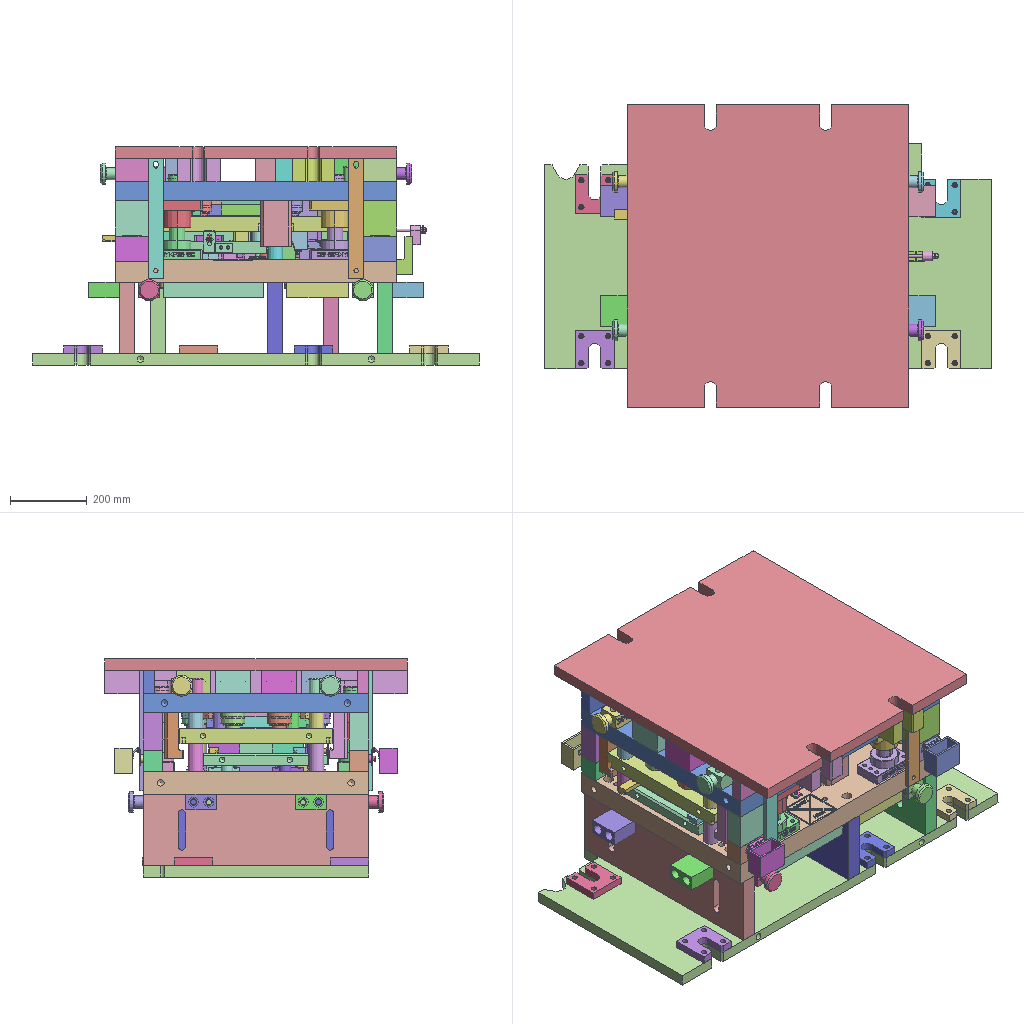Assembly | STEP file | 487 different items | 487 placed | box 1160 x 785 x 567 mm
Parts list (item | name | quantity | size | volume):
1 | 13001_id1154_x_t | x1 | 730 x 585 x 50 mm | 18693036 mm3
2 | 13101_id1802_x_t | x1 | 85 x 30 x 60 mm | 133679 mm3
3 | 13101_id1806_x_t | x1 | 85 x 30 x 60 mm | 133679 mm3
4 | 13101_id1810_x_t | x1 | 85 x 30 x 60 mm | 133679 mm3
5 | 13101_id1814_x_t | x1 | 85 x 30 x 60 mm | 133679 mm3
6 | 13102_id1494_x_t | x1 | 90 x 90 x 60 mm | 430512 mm3
7 | 13102_id1498_x_t | x1 | 90 x 90 x 60 mm | 430512 mm3
8 | 13103_id1506_x_t | x1 | 30 x 90 x 60 mm | 142679 mm3
9 | 13104_id1502_x_t | x1 | 25 x 90 x 60 mm | 115679 mm3
10 | 13105_id1770_x_t | x1 | 112 x 785 x 60 mm | 4657225 mm3
11 | 13106_id1778_x_t | x1 | 90 x 90 x 60 mm | 428886 mm3
12 | 13106_id1782_x_t | x1 | 90 x 90 x 60 mm | 428886 mm3
13 | 13106_id1786_x_t | x1 | 90 x 90 x 60 mm | 428886 mm3
14 | 13106_id1790_x_t | x1 | 90 x 90 x 60 mm | 428886 mm3
15 | 13106_id1794_x_t | x1 | 90 x 90 x 60 mm | 428886 mm3
16 | 13106_id1798_x_t | x1 | 90 x 90 x 60 mm | 428886 mm3
17 | 13107_id1774_x_t | x1 | 110 x 785 x 60 mm | 3912002 mm3
18 | 14001_id1214_x_t | x1 | 40 x 40 x 40 mm | 44485 mm3
19 | 14001_id1218_x_t | x1 | 40 x 40 x 40 mm | 44485 mm3
20 | 14001_id1222_x_t | x1 | 40 x 40 x 40 mm | 44485 mm3
21 | 14001_id1226_x_t | x1 | 40 x 40 x 40 mm | 44485 mm3
22 | 14001_id1230_x_t | x1 | 40 x 40 x 40 mm | 44485 mm3
23 | 14001_id1234_x_t | x1 | 40 x 40 x 40 mm | 44485 mm3
24 | 14001_id1238_x_t | x1 | 40 x 40 x 40 mm | 44485 mm3
25 | 14001_id1242_x_t | x1 | 40 x 40 x 40 mm | 44485 mm3
26 | 14001_id1246_x_t | x1 | 40 x 40 x 40 mm | 44485 mm3
27 | 14001_id1250_x_t | x1 | 40 x 40 x 40 mm | 44485 mm3
28 | 14001_id1254_x_t | x1 | 40 x 40 x 40 mm | 44485 mm3
29 | 14001_id1258_x_t | x1 | 40 x 40 x 40 mm | 44485 mm3
30 | 14001_id1262_x_t | x1 | 40 x 40 x 40 mm | 44485 mm3
31 | 14001_id1266_x_t | x1 | 40 x 40 x 40 mm | 44485 mm3
32 | 14001_id1298_x_t | x1 | 40 x 40 x 40 mm | 44485 mm3
33 | 14001_id1306_x_t | x1 | 40 x 40 x 40 mm | 44485 mm3
34 | 14002_id1738_x_t | x1 | 30.406 x 30.406 x 15 mm | 5664 mm3
35 | 14002_id1742_x_t | x1 | 30.406 x 30.406 x 15 mm | 5664 mm3
36 | 14002_id1746_x_t | x1 | 28.807 x 23.857 x 15 mm | 5664 mm3
37 | 14002_id1750_x_t | x1 | 28.807 x 23.857 x 15 mm | 5664 mm3
38 | 14002_id1754_x_t | x1 | 27.746 x 22.068 x 15 mm | 5664 mm3
39 | 14002_id1758_x_t | x1 | 27.746 x 22.068 x 15 mm | 5664 mm3
40 | 14002_id1762_x_t | x1 | 29.858 x 30.721 x 15 mm | 5664 mm3
41 | 14002_id1766_x_t | x1 | 29.858 x 30.721 x 15 mm | 5664 mm3
42 | 14003_id1942_x_t | x1 | 30 x 16 x 16 mm | 6162 mm3
43 | 14004_id1938_x_t | x1 | 30 x 16 x 16 mm | 6162 mm3
44 | 14101_id882_x_t | x1 | 25 x 40 x 50 mm | 37635 mm3
45 | 14102_id878_x_t | x1 | 25 x 40 x 50 mm | 37635 mm3
46 | 14103_id870_x_t | x1 | 95 x 130 x 28 mm | 241686 mm3
47 | 14104_id886_x_t | x1 | 40 x 25 x 50 mm | 37460 mm3
48 | 14105_id890_x_t | x1 | 90 x 75 x 28 mm | 120807 mm3
49 | 14106_id898_x_t | x1 | 43 x 30 x 50 mm | 41594 mm3
50 | 14107_id966_x_t | x1 | 105 x 120 x 28 mm | 217134 mm3
51 | 14108_id962_x_t | x1 | 105 x 120 x 28 mm | 217134 mm3
52 | 14109_id1038_x_t | x1 | 51 x 55 x 50 mm | 79399 mm3
53 | 14110_id1022_x_t | x1 | 105 x 176 x 28 mm | 281247 mm3
54 | 14111_id1006_x_t | x1 | 51 x 55 x 50 mm | 79567 mm3
55 | 14112_id1034_x_t | x1 | 60 x 85 x 28 mm | 85179 mm3
56 | 14113_id846_x_t | x1 | 727.5 x 395 x 40 mm | 9281090 mm3
57 | 15001_id142_x_t | x1 | 15 x 17 x 108 mm | 21787 mm3
58 | 15002_id766_x_t | x1 | 48.641 x 98 x 108 mm | 278629 mm3
59 | 15003_id762_x_t | x1 | 48.641 x 98 x 108 mm | 278628 mm3
60 | 15004_id854_x_t | x1 | 51.676 x 85.003 x 65 mm | 145640 mm3
61 | 15005_id190_x_t | x1 | 51.676 x 85 x 65 mm | 145641 mm3
62 | 15006_id866_x_t | x1 | 42.5 x 42 x 101 mm | 91343 mm3
63 | 15101_id1058_x_t | x1 | 63.914 x 80 x 35 mm | 137778 mm3
64 | 15102_id758_x_t | x1 | 63.914 x 80 x 35 mm | 137778 mm3
65 | 15103_id754_x_t | x1 | 290 x 208 x 25 mm | 1200558 mm3
66 | 15104_id194_x_t | x1 | 50.466 x 210 x 37 mm | 295873 mm3
67 | 15105_id234_x_t | x1 | 149.23 x 42 x 25 mm | 138214 mm3
68 | 15106_id1078_x_t | x1 | 70 x 85 x 53 mm | 208410 mm3
69 | 15107_id1946_x_t | x1 | 70 x 85 x 53 mm | 208411 mm3
70 | 15108_id850_x_t | x1 | 115 x 175 x 25 mm | 409284 mm3
71 | 16001_id1410_x_t | x1 | 85 x 50 x 97 mm | 372174 mm3
72 | 16001_id1450_x_t | x1 | 85 x 50 x 97 mm | 372174 mm3
73 | 16001_id1466_x_t | x1 | 85 x 50 x 97 mm | 372174 mm3
74 | 16001_id1482_x_t | x1 | 85 x 50 x 97 mm | 372174 mm3
75 | 16002_id1274_x_t | x1 | 80 x 50 x 118 mm | 264145 mm3
76 | 16002_id1278_x_t | x1 | 80 x 50 x 118 mm | 264145 mm3
77 | 16002_id1282_x_t | x1 | 80 x 50 x 118 mm | 264145 mm3
78 | 16002_id1286_x_t | x1 | 80 x 50 x 118 mm | 264145 mm3
79 | 16002_id1290_x_t | x1 | 80 x 50 x 118 mm | 264145 mm3
80 | 16002_id1294_x_t | x1 | 80 x 50 x 118 mm | 264145 mm3
81 | 16003_id874_x_t | x1 | 95 x 130 x 10 mm | 115889 mm3
82 | 16004_id894_x_t | x1 | 90 x 75 x 10 mm | 57234 mm3
83 | 16005_id970_x_t | x1 | 105 x 120 x 10 mm | 118397 mm3
84 | 16005_id974_x_t | x1 | 105 x 120 x 10 mm | 118397 mm3
85 | 16006_id862_x_t | x1 | 74.676 x 85 x 110 mm | 490058 mm3
86 | 16007_id858_x_t | x1 | 74.676 x 85 x 110 mm | 490062 mm3
87 | 16008_id1026_x_t | x1 | 105 x 176 x 10 mm | 142706 mm3
88 | 16009_id1030_x_t | x1 | 60 x 85 x 10 mm | 42512 mm3
89 | 6-35_id1850_x_t | x1 | 8 x 8 x 38 mm | 1137 mm3
90 | 6-35_id1870_x_t | x1 | 8 x 8 x 38 mm | 1137 mm3
91 | - | x1 | 94 x 140 x 15 mm | 130830 mm3
92 | - | x1 | 58 x 85.001 x 56.5 mm | 200915 mm3
93 | - | x1 | 30 x 30 x 27 mm | 14276 mm3
94 | - | x1 | 30 x 30 x 27 mm | 14276 mm3
95 | - | x1 | 30 x 30 x 27 mm | 14276 mm3
96 | - | x1 | 26.045 x 93.231 x 17.45 mm | 4101 mm3
97 | - | x1 | 30 x 30 x 27 mm | 14276 mm3
98 | - | x1 | 40 x 40 x 72 mm | 79413 mm3
99 | - | x1 | 40 x 40 x 72 mm | 79413 mm3
100 | - | x1 | 40 x 40 x 72 mm | 79413 mm3
101 | - | x1 | 40 x 40 x 72 mm | 79413 mm3
102 | - | x1 | 99 x 140 x 30 mm | 280871 mm3
103 | - | x1 | 40 x 40 x 72 mm | 79413 mm3
104 | - | x1 | 99 x 140 x 15 mm | 135777 mm3
105 | - | x1 | 40 x 40 x 72 mm | 79413 mm3
106 | - | x1 | 42 x 25 x 98 mm | 60681 mm3
107 | - | x1 | 40 x 585 x 185 mm | 4078797 mm3
108 | - | x1 | 40 x 585 x 185 mm | 4012325 mm3
109 | - | x1 | 100 x 100 x 20 mm | 150755 mm3
110 | - | x1 | 100 x 100 x 20 mm | 150755 mm3
111 | - | x1 | 100 x 100 x 20 mm | 150755 mm3
112 | - | x1 | 40 x 255 x 185 mm | 1855337 mm3
113 | - | x1 | 40 x 255 x 185 mm | 1874377 mm3
114 | - | x1 | 40 x 585 x 185 mm | 4281820 mm3
115 | - | x1 | 85 x 50 x 55 mm | 210302 mm3
116 | - | x1 | 85 x 74 x 66.5 mm | 93814 mm3
117 | - | x1 | 85 x 50 x 55 mm | 210302 mm3
118 | - | x1 | 85 x 74 x 66.5 mm | 93814 mm3
119 | - | x1 | 85 x 50 x 55 mm | 210302 mm3
120 | - | x1 | 63 x 73 x 30 mm | 93374 mm3
121 | - | x1 | 85 x 74 x 66.5 mm | 93814 mm3
122 | - | x1 | 85 x 50 x 55 mm | 210302 mm3
123 | - | x1 | 85 x 74 x 66.5 mm | 93814 mm3
124 | - | x1 | 60 x 80 x 56.5 mm | 99207 mm3
125 | - | x1 | 28 x 43 x 30 mm | 25680 mm3
126 | - | x1 | 63 x 73 x 15 mm | 59595 mm3
127 | - | x1 | 30 x 30 x 15 mm | 8745 mm3
128 | - | x1 | 30 x 30 x 15 mm | 8745 mm3
129 | - | x1 | 30 x 30 x 15 mm | 8745 mm3
130 | - | x1 | 30 x 30 x 15 mm | 8745 mm3
131 | - | x1 | 30 x 30 x 15 mm | 8745 mm3
132 | - | x1 | 105 x 25 x 16 mm | 33608 mm3
133 | - | x1 | 45 x 25 x 16 mm | 13030 mm3
134 | - | x1 | 90 x 25 x 80 mm | 146448 mm3
135 | - | x1 | 90 x 25 x 80 mm | 146448 mm3
136 | - | x1 | 80 x 80 x 40 mm | 195367 mm3
137 | - | x1 | 80 x 80 x 40 mm | 195367 mm3
138 | - | x1 | 80 x 80 x 40 mm | 195367 mm3
139 | - | x1 | 80 x 80 x 40 mm | 195367 mm3
140 | - | x1 | 19.63 x 48.1 x 17 mm | 5552 mm3
141 | - | x1 | 75 x 27 x 53.7 mm | 8311 mm3
142 | - | x1 | 65 x 48 x 16 mm | 32002 mm3
143 | - | x1 | 15 x 70.5 x 16 mm | 11235 mm3
144 | - | x1 | 1160 x 585 x 30 mm | 18789042 mm3
145 | - | x1 | 100 x 100 x 20 mm | 150755 mm3
146 | - | x1 | 100 x 100 x 20 mm | 150755 mm3
147 | - | x1 | 19.1 x 19.1 x 30 mm | 8502 mm3
148 | - | x1 | 260 x 40 x 40 mm | 385684 mm3
149 | - | x1 | 260 x 40 x 40 mm | 385684 mm3
150 | - | x1 | 160 x 40 x 40 mm | 225684 mm3
151 | - | x1 | 160 x 40 x 40 mm | 225684 mm3
152 | - | x1 | 100 x 100 x 20 mm | 150755 mm3
153 | - | x1 | 40 x 10 x 317 mm | 124006 mm3
154 | - | x1 | 40 x 10 x 317 mm | 124006 mm3
155 | - | x1 | 40 x 10 x 317 mm | 124006 mm3
156 | - | x1 | 40 x 10 x 317 mm | 124006 mm3
157 | - | x1 | 58.148 x 85 x 56.5 mm | 200916 mm3
158 | - | x1 | 58 x 85 x 56.501 mm | 217515 mm3
159 | - | x1 | 40 x 55 x 53 mm | 73845 mm3
160 | - | x1 | - | 214872 mm3
161 | - | x1 | 65 x 75 x 45.001 mm | 106035 mm3
162 | - | x1 | 19 x 17 x 20 mm | 5075 mm3
163 | - | x1 | 15 x 13 x 20 mm | 2634 mm3
164 | - | x1 | 13.98 x 12 x 20 mm | 2357 mm3
165 | - | x1 | 23.1 x 23.1 x 30 mm | 13334 mm3
166 | - | x1 | 80 x 90 x 30 mm | 141495 mm3
167 | - | x1 | 80 x 90 x 15 mm | 69642 mm3
168 | - | x1 | 70 x 120 x 30 mm | 188611 mm3
169 | - | x1 | 40 x 55 x 53 mm | 73845 mm3
170 | - | x1 | 58 x 85 x 56.501 mm | 217785 mm3
171 | - | x1 | 70 x 120 x 15 mm | 114867 mm3
172 | - | x1 | 58.914 x 80 x 15 mm | 42146 mm3
173 | - | x1 | 19.1 x 19.1 x 30 mm | 8502 mm3
174 | - | x1 | 60 x 80 x 56.5 mm | 99206 mm3
175 | - | x1 | 58.914 x 80 x 15 mm | 42146 mm3
176 | - | x1 | 105 x 25 x 16 mm | 33608 mm3
177 | - | x1 | 70 x 33 x 16 mm | 29565 mm3
178 | - | x1 | 20 x 25 x 7 mm | 3055 mm3
179 | - | x1 | 20 x 25 x 7 mm | 3055 mm3
180 | - | x1 | 20 x 25 x 7 mm | 3055 mm3
181 | - | x1 | 25 x 20 x 7 mm | 3055 mm3
182 | - | x1 | 730 x 585 x 60 mm | 23773121 mm3
183 | - | x1 | 240 x 52 x 30 mm | 250447 mm3
184 | - | x1 | 65 x 75 x 45.001 mm | 106042 mm3
185 | - | x1 | 19 x 17 x 20 mm | 5075 mm3
186 | - | x1 | 15 x 13 x 20 mm | 2634 mm3
187 | - | x1 | 13.98 x 12 x 20 mm | 2357 mm3
188 | - | x1 | 730 x 785 x 30 mm | 16951245 mm3
189 | - | x1 | 20 x 25 x 7 mm | 3055 mm3
190 | - | x1 | 25 x 20 x 7 mm | 3055 mm3
191 | - | x1 | 94 x 140 x 30 mm | 271163 mm3
192 | - | x1 | 400 x 325 x 30 mm | 2323925 mm3
193 | CB-_id1538_x_t | x1 | 16 x 16 x 50 mm | 4584 mm3
194 | CB-_id1542_x_t | x1 | 16 x 16 x 50 mm | 4584 mm3
195 | CB-_id1558_x_t | x1 | 16 x 16 x 50 mm | 4584 mm3
196 | CB-_id1562_x_t | x1 | 16 x 16 x 50 mm | 4584 mm3
197 | CHP10_id1818_x_t | x1 | 118 x 55 x 55 mm | 202286 mm3
198 | CHP10_id1822_x_t | x1 | 118 x 55 x 55 mm | 202286 mm3
199 | CHP10_id1826_x_t | x1 | 118 x 55 x 55 mm | 202286 mm3
200 | CHP10_id1830_x_t | x1 | 118 x 55 x 55 mm | 202286 mm3
201 | CHP10_id1834_x_t | x1 | 55 x 118 x 55 mm | 202286 mm3
202 | CHP10_id1838_x_t | x1 | 55 x 118 x 55 mm | 202286 mm3
203 | CHP10_id1842_x_t | x1 | 55 x 118 x 55 mm | 202286 mm3
204 | CHP10_id1846_x_t | x1 | 55 x 118 x 55 mm | 202286 mm3
205 | D10-50_id1526_x_t | x1 | 10 x 10 x 50 mm | 3878 mm3
206 | D10-50_id1546_x_t | x1 | 10 x 10 x 50 mm | 3878 mm3
207 | D10-50_id1566_x_t | x1 | 10 x 10 x 50 mm | 3878 mm3
208 | D8-50_id110_x_t | x1 | 10 x 10 x 50 mm | 3919 mm3
209 | D8-50_id114_x_t | x1 | 10 x 10 x 50 mm | 3919 mm3
210 | D8-50_id118_x_t | x1 | 10 x 10 x 50 mm | 3919 mm3
211 | D8-50_id122_x_t | x1 | 10 x 10 x 50 mm | 3919 mm3
212 | D8-50_id1614_x_t | x1 | 8 x 8 x 30 mm | 1502 mm3
213 | D8-50_id1622_x_t | x1 | 8 x 8 x 30 mm | 1502 mm3
214 | D8-50_id1634_x_t | x1 | 8 x 8 x 30 mm | 1502 mm3
215 | D8-50_id1642_x_t | x1 | 8 x 8 x 30 mm | 1502 mm3
216 | D8-50_id1654_x_t | x1 | 8 x 8 x 30 mm | 1502 mm3
217 | D8-50_id1658_x_t | x1 | 8 x 8 x 30 mm | 1502 mm3
218 | D8-50_id1662_x_t | x1 | 8 x 8 x 30 mm | 1502 mm3
219 | D8-50_id166_x_t | x1 | 8 x 8 x 45 mm | 2256 mm3
220 | D8-50_id1674_x_t | x1 | 8 x 8 x 30 mm | 1502 mm3
221 | D8-50_id1686_x_t | x1 | 8 x 8 x 30 mm | 1502 mm3
222 | D8-50_id1690_x_t | x1 | 8 x 8 x 30 mm | 1502 mm3
223 | D8-50_id170_x_t | x1 | 8 x 8 x 45 mm | 2256 mm3
224 | D8-50_id294_x_t | x1 | 8 x 8 x 30 mm | 1502 mm3
225 | D8-50_id298_x_t | x1 | 8 x 8 x 30 mm | 1502 mm3
226 | D8-50_id354_x_t | x1 | 8 x 8 x 45 mm | 2256 mm3
227 | D8-50_id362_x_t | x1 | 8 x 8 x 45 mm | 2256 mm3
228 | D8-50_id394_x_t | x1 | 8 x 8 x 30 mm | 1502 mm3
229 | D8-50_id398_x_t | x1 | 8 x 8 x 30 mm | 1502 mm3
230 | D8-50_id406_x_t | x1 | 10 x 10 x 40 mm | 3134 mm3
231 | D8-50_id410_x_t | x1 | 8 x 8 x 30 mm | 1502 mm3
232 | D8-50_id426_x_t | x1 | 8 x 8 x 30 mm | 1502 mm3
233 | D8-50_id446_x_t | x1 | 10 x 10 x 40 mm | 3134 mm3
234 | D8-50_id474_x_t | x1 | 8 x 8 x 30 mm | 1502 mm3
235 | D8-50_id478_x_t | x1 | 8 x 8 x 30 mm | 1502 mm3
236 | D8-50_id486_x_t | x1 | 8 x 8 x 30 mm | 1502 mm3
237 | D8-50_id490_x_t | x1 | 8 x 8 x 30 mm | 1502 mm3
238 | D8-50_id54_x_t | x1 | 10 x 10 x 50 mm | 3919 mm3
239 | D8-50_id622_x_t | x1 | 8 x 8 x 30 mm | 1502 mm3
240 | D8-50_id626_x_t | x1 | 8 x 8 x 30 mm | 1502 mm3
241 | D8-50_id62_x_t | x1 | 10 x 10 x 50 mm | 3919 mm3
242 | D8-50_id82_x_t | x1 | 10 x 10 x 40 mm | 3134 mm3
243 | D8-50_id86_x_t | x1 | 10 x 10 x 40 mm | 3134 mm3
244 | GSV170-7_id1158_x_t | x1 | 50 x 50 x 114 mm | 158224 mm3
245 | GSV170-7_id1162_x_t | x1 | 50 x 50 x 114 mm | 158224 mm3
246 | GSV170-7_id1166_x_t | x1 | 50 x 50 x 114 mm | 158224 mm3
247 | GSV170-7_id1170_x_t | x1 | 50 x 50 x 114 mm | 158224 mm3
248 | GSV170-7_id1174_x_t | x1 | 50 x 50 x 114 mm | 158224 mm3
249 | GSV170-7_id1178_x_t | x1 | 50 x 50 x 114 mm | 158224 mm3
250 | GSV170-7_id1182_x_t | x1 | 63 x 63 x 120 mm | 273871 mm3
251 | GSV170-7_id1186_x_t | x1 | 63 x 63 x 120 mm | 273871 mm3
252 | GSV170-7_id1190_x_t | x1 | 63 x 63 x 120 mm | 273871 mm3
253 | GSV170-7_id1194_x_t | x1 | 63 x 63 x 120 mm | 273871 mm3
254 | GSV170-7_id1270_x_t | x1 | 50 x 50 x 114 mm | 158224 mm3
255 | GSV170-7_id506_x_t | x1 | 19 x 19 x 106 mm | 21365 mm3
256 | GSV170-7_id514_x_t | x1 | 19 x 19 x 106 mm | 21365 mm3
257 | GSV170-7_id530_x_t | x1 | 19 x 19 x 106 mm | 21365 mm3
258 | GSV170-7_id550_x_t | x1 | 19 x 19 x 106 mm | 21365 mm3
259 | GSV170-7_id670_x_t | x1 | 19 x 19 x 106 mm | 21365 mm3
260 | GSV170-7_id734_x_t | x1 | 19 x 19 x 106 mm | 21365 mm3
261 | LPS 2-10_id1002_x_t | x1 | 8 x 8 x 60 mm | 2567 mm3
262 | LPS 2-10_id1010_x_t | x1 | 8 x 8 x 60 mm | 2567 mm3
263 | LPS 2-10_id1014_x_t | x1 | 8 x 8 x 60 mm | 2567 mm3
264 | LPS 2-10_id1018_x_t | x1 | 8 x 8 x 60 mm | 2567 mm3
265 | LPS 2-10_id1042_x_t | x1 | 8 x 8 x 60 mm | 2567 mm3
266 | LPS 2-10_id1046_x_t | x1 | 8 x 8 x 60 mm | 2567 mm3
267 | LPS 2-10_id1050_x_t | x1 | 8 x 8 x 60 mm | 2567 mm3
268 | LPS 2-10_id1054_x_t | x1 | 8 x 8 x 60 mm | 2567 mm3
269 | LPS 2-10_id902_x_t | x1 | 8 x 8 x 60 mm | 2567 mm3
270 | LPS 2-10_id906_x_t | x1 | 8 x 8 x 60 mm | 2567 mm3
271 | LPS 2-10_id910_x_t | x1 | 8 x 8 x 60 mm | 2567 mm3
272 | LPS 2-10_id914_x_t | x1 | 8 x 8 x 60 mm | 2567 mm3
273 | LPS 2-10_id918_x_t | x1 | 8 x 8 x 60 mm | 2567 mm3
274 | LPS 2-10_id922_x_t | x1 | 8 x 8 x 60 mm | 2567 mm3
275 | LPS 2-10_id926_x_t | x1 | 8 x 8 x 60 mm | 2567 mm3
276 | LPS 2-10_id930_x_t | x1 | 8 x 8 x 60 mm | 2567 mm3
277 | LPS 2-10_id934_x_t | x1 | 8 x 8 x 60 mm | 2567 mm3
278 | LPS 2-10_id938_x_t | x1 | 8 x 8 x 60 mm | 2567 mm3
279 | LPS 2-10_id942_x_t | x1 | 8 x 8 x 60 mm | 2567 mm3
280 | LPS 2-10_id946_x_t | x1 | 8 x 8 x 60 mm | 2567 mm3
281 | LPS 2-10_id950_x_t | x1 | 8 x 8 x 60 mm | 2567 mm3
282 | LPS 2-10_id954_x_t | x1 | 8 x 8 x 60 mm | 2567 mm3
283 | LPS 2-10_id958_x_t | x1 | 8 x 8 x 60 mm | 2567 mm3
284 | LPS 2-10_id978_x_t | x1 | 8 x 8 x 60 mm | 2567 mm3
285 | LPS 2-10_id982_x_t | x1 | 8 x 8 x 60 mm | 2567 mm3
286 | LPS 2-10_id986_x_t | x1 | 8 x 8 x 60 mm | 2567 mm3
287 | LPS 2-10_id990_x_t | x1 | 8 x 8 x 60 mm | 2567 mm3
288 | LPS 2-10_id994_x_t | x1 | 8 x 8 x 60 mm | 2567 mm3
289 | LPS 2-10_id998_x_t | x1 | 8 x 8 x 60 mm | 2567 mm3
290 | M3-10_id102_x_t | x1 | 16 x 16 x 55 mm | 4808 mm3
291 | M3-10_id134_x_t | x1 | 16 x 16 x 55 mm | 4808 mm3
292 | M3-10_id1370_x_t | x1 | 43 x 13 x 13 mm | 2482 mm3
293 | M3-10_id138_x_t | x1 | 16 x 16 x 55 mm | 4808 mm3
294 | M3-10_id1418_x_t | x1 | 16 x 16 x 45 mm | 4022 mm3
295 | M3-10_id1422_x_t | x1 | 16 x 16 x 45 mm | 4022 mm3
296 | M3-10_id1426_x_t | x1 | 13 x 33 x 13 mm | 1987 mm3
297 | M3-10_id1430_x_t | x1 | 13 x 33 x 13 mm | 1987 mm3
298 | M3-10_id1438_x_t | x1 | 16 x 16 x 45 mm | 4022 mm3
299 | M3-10_id1442_x_t | x1 | 13 x 33 x 13 mm | 1987 mm3
300 | M3-10_id1446_x_t | x1 | 13 x 33 x 13 mm | 1987 mm3
301 | M3-10_id1458_x_t | x1 | 16 x 16 x 45 mm | 4022 mm3
302 | M3-10_id1478_x_t | x1 | 16 x 16 x 45 mm | 4022 mm3
303 | M3-10_id1490_x_t | x1 | 16 x 16 x 45 mm | 4022 mm3
304 | M3-10_id1574_x_t | x1 | 13 x 13 x 28 mm | 1728 mm3
305 | M3-10_id1582_x_t | x1 | 13 x 13 x 28 mm | 1728 mm3
306 | M3-10_id1586_x_t | x1 | 13 x 13 x 28 mm | 1728 mm3
307 | M3-10_id158_x_t | x1 | 13 x 13 x 48 mm | 2734 mm3
308 | M3-10_id1598_x_t | x1 | 13 x 13 x 28 mm | 1728 mm3
309 | M3-10_id1606_x_t | x1 | 13 x 13 x 28 mm | 1728 mm3
310 | M3-10_id1618_x_t | x1 | 13 x 13 x 28 mm | 1742 mm3
311 | M3-10_id1626_x_t | x1 | 13 x 13 x 28 mm | 1742 mm3
312 | M3-10_id162_x_t | x1 | 13 x 13 x 48 mm | 2734 mm3
313 | M3-10_id1638_x_t | x1 | 13 x 13 x 28 mm | 1742 mm3
314 | M3-10_id1650_x_t | x1 | 13 x 13 x 48 mm | 2734 mm3
315 | M3-10_id1666_x_t | x1 | 13 x 13 x 48 mm | 2734 mm3
316 | M3-10_id1678_x_t | x1 | 13 x 13 x 28 mm | 1742 mm3
317 | M3-10_id1682_x_t | x1 | 13 x 13 x 28 mm | 1742 mm3
318 | M3-10_id210_x_t | x1 | 20 x 8.5 x 8.5 mm | 482.387 mm3
319 | M3-10_id214_x_t | x1 | 20 x 8.5 x 8.5 mm | 482.387 mm3
320 | M3-10_id218_x_t | x1 | 16 x 16 x 40 mm | 3630 mm3
321 | M3-10_id222_x_t | x1 | 16 x 16 x 40 mm | 3630 mm3
322 | M3-10_id226_x_t | x1 | 16 x 16 x 40 mm | 3630 mm3
323 | M3-10_id230_x_t | x1 | 16 x 16 x 40 mm | 3630 mm3
324 | M3-10_id238_x_t | x1 | 16 x 16 x 40 mm | 3630 mm3
325 | M3-10_id242_x_t | x1 | 16 x 16 x 40 mm | 3630 mm3
326 | M3-10_id262_x_t | x1 | 8.5 x 8.5 x 20 mm | 456.375 mm3
327 | M3-10_id266_x_t | x1 | 8.5 x 8.5 x 20 mm | 456.375 mm3
328 | M3-10_id270_x_t | x1 | 8.5 x 8.5 x 20 mm | 456.375 mm3
329 | M3-10_id278_x_t | x1 | 10 x 10 x 46 mm | 1459 mm3
330 | M3-10_id282_x_t | x1 | 13 x 13 x 33 mm | 1980 mm3
331 | M3-10_id286_x_t | x1 | 13 x 13 x 33 mm | 1980 mm3
332 | M3-10_id290_x_t | x1 | 13 x 13 x 33 mm | 1980 mm3
333 | M3-10_id306_x_t | x1 | 20 x 8.5 x 8.5 mm | 482.387 mm3
334 | M3-10_id310_x_t | x1 | 16 x 16 x 40 mm | 3630 mm3
335 | M3-10_id314_x_t | x1 | 16 x 16 x 40 mm | 3630 mm3
336 | M3-10_id318_x_t | x1 | 20 x 8.5 x 8.5 mm | 482.387 mm3
337 | M3-10_id322_x_t | x1 | 16 x 16 x 40 mm | 3630 mm3
338 | M3-10_id326_x_t | x1 | 16 x 16 x 40 mm | 3630 mm3
339 | M3-10_id338_x_t | x1 | 16 x 16 x 40 mm | 3630 mm3
340 | M3-10_id346_x_t | x1 | 16 x 16 x 40 mm | 3630 mm3
341 | M3-10_id350_x_t | x1 | 13 x 13 x 48 mm | 2734 mm3
342 | M3-10_id358_x_t | x1 | 13 x 13 x 48 mm | 2734 mm3
343 | M3-10_id374_x_t | x1 | 8.5 x 8.5 x 20 mm | 456.375 mm3
344 | M3-10_id378_x_t | x1 | 13 x 13 x 28 mm | 1728 mm3
345 | M3-10_id382_x_t | x1 | 13 x 13 x 28 mm | 1728 mm3
346 | M3-10_id386_x_t | x1 | 13 x 13 x 28 mm | 1728 mm3
347 | M3-10_id38_x_t | x1 | 8.5 x 8.5 x 20 mm | 456.375 mm3
348 | M3-10_id390_x_t | x1 | 13 x 13 x 28 mm | 1728 mm3
349 | M3-10_id402_x_t | x1 | 13 x 13 x 28 mm | 1728 mm3
350 | M3-10_id414_x_t | x1 | 13 x 13 x 33 mm | 1980 mm3
351 | M3-10_id418_x_t | x1 | 13 x 13 x 33 mm | 1980 mm3
352 | M3-10_id422_x_t | x1 | 13 x 13 x 28 mm | 1728 mm3
353 | M3-10_id42_x_t | x1 | 8.5 x 8.5 x 20 mm | 456.375 mm3
354 | M3-10_id434_x_t | x1 | 13 x 13 x 33 mm | 1980 mm3
355 | M3-10_id442_x_t | x1 | 13 x 13 x 28 mm | 1728 mm3
356 | M3-10_id450_x_t | x1 | 13 x 13 x 28 mm | 1728 mm3
357 | M3-10_id454_x_t | x1 | 13 x 13 x 33 mm | 1980 mm3
358 | M3-10_id466_x_t | x1 | 13 x 13 x 28 mm | 1742 mm3
359 | M3-10_id46_x_t | x1 | 16 x 16 x 55 mm | 4808 mm3
360 | M3-10_id470_x_t | x1 | 13 x 13 x 28 mm | 1742 mm3
361 | M3-10_id482_x_t | x1 | 13 x 13 x 28 mm | 1742 mm3
362 | M3-10_id50_x_t | x1 | 16 x 16 x 55 mm | 4808 mm3
363 | M3-10_id566_x_t | x1 | 10 x 10 x 26 mm | 877.848 mm3
364 | M3-10_id570_x_t | x1 | 10 x 10 x 26 mm | 877.848 mm3
365 | M3-10_id574_x_t | x1 | 10 x 10 x 26 mm | 877.848 mm3
366 | M3-10_id578_x_t | x1 | 10 x 10 x 26 mm | 877.848 mm3
367 | M3-10_id582_x_t | x1 | 10 x 10 x 26 mm | 877.848 mm3
368 | M3-10_id586_x_t | x1 | 10 x 10 x 26 mm | 877.848 mm3
369 | M3-10_id58_x_t | x1 | 16 x 16 x 55 mm | 4808 mm3
370 | M3-10_id590_x_t | x1 | 10 x 10 x 26 mm | 877.848 mm3
371 | M3-10_id594_x_t | x1 | 10 x 10 x 26 mm | 877.848 mm3
372 | M3-10_id598_x_t | x1 | 13 x 13 x 28 mm | 1756 mm3
373 | M3-10_id602_x_t | x1 | 13 x 13 x 28 mm | 1756 mm3
374 | M3-10_id606_x_t | x1 | 13 x 13 x 28 mm | 1756 mm3
375 | M3-10_id614_x_t | x1 | 8.5 x 8.5 x 20 mm | 456.375 mm3
376 | M3-10_id630_x_t | x1 | 13 x 13 x 33 mm | 1980 mm3
377 | M3-10_id634_x_t | x1 | 8.5 x 8.5 x 20 mm | 456.375 mm3
378 | M3-10_id638_x_t | x1 | 8.5 x 8.5 x 20 mm | 456.375 mm3
379 | M3-10_id646_x_t | x1 | 13 x 13 x 33 mm | 1980 mm3
380 | M3-10_id658_x_t | x1 | 13 x 13 x 33 mm | 1980 mm3
381 | M3-10_id662_x_t | x1 | 10 x 10 x 26 mm | 877.848 mm3
382 | M3-10_id666_x_t | x1 | 10 x 10 x 26 mm | 877.848 mm3
383 | M3-10_id66_x_t | x1 | 13 x 13 x 33 mm | 1980 mm3
384 | M3-10_id678_x_t | x1 | 13 x 13 x 33 mm | 1980 mm3
385 | M3-10_id682_x_t | x1 | 13 x 13 x 33 mm | 1980 mm3
386 | M3-10_id686_x_t | x1 | 13 x 13 x 33 mm | 1980 mm3
387 | M3-10_id690_x_t | x1 | 13 x 13 x 33 mm | 1980 mm3
388 | M3-10_id698_x_t | x1 | 13 x 13 x 33 mm | 1980 mm3
389 | M3-10_id706_x_t | x1 | 13 x 13 x 28 mm | 1756 mm3
390 | M3-10_id70_x_t | x1 | 13 x 13 x 33 mm | 1980 mm3
391 | M3-10_id710_x_t | x1 | 10 x 10 x 26 mm | 877.848 mm3
392 | M3-10_id714_x_t | x1 | 10 x 10 x 26 mm | 877.848 mm3
393 | M3-10_id718_x_t | x1 | 13 x 13 x 28 mm | 1756 mm3
394 | M3-10_id742_x_t | x1 | 13 x 13 x 33 mm | 1980 mm3
395 | M3-10_id74_x_t | x1 | 13 x 13 x 33 mm | 1980 mm3
396 | M3-10_id78_x_t | x1 | 13 x 13 x 33 mm | 1980 mm3
397 | M3-10_id98_x_t | x1 | 16 x 16 x 55 mm | 4808 mm3
398 | M6-40_id1086_x_t | x1 | 16 x 16 x 40 mm | 3648 mm3
399 | M6-40_id1094_x_t | x1 | 16 x 16 x 40 mm | 3648 mm3
400 | M6-40_id1102_x_t | x1 | 16 x 16 x 40 mm | 3648 mm3
401 | M6-40_id1110_x_t | x1 | 16 x 16 x 40 mm | 3648 mm3
402 | M6-40_id1118_x_t | x1 | 16 x 16 x 70 mm | 6004 mm3
403 | M6-40_id1126_x_t | x1 | 16 x 16 x 70 mm | 6004 mm3
404 | M6-40_id1130_x_t | x1 | 16 x 16 x 70 mm | 6004 mm3
405 | M6-40_id1134_x_t | x1 | 16 x 16 x 70 mm | 6004 mm3
406 | M6-40_id1142_x_t | x1 | 16 x 16 x 70 mm | 6004 mm3
407 | M6-40_id1150_x_t | x1 | 16 x 16 x 70 mm | 6004 mm3
408 | MI_APAL_0099_id1062_x_t | x1 | 13 x 13 x 100 mm | 5213 mm3
409 | MI_APAL_0099_id1066_x_t | x1 | 13 x 13 x 100 mm | 5213 mm3
410 | MI_APAL_0100_id1070_x_t | x1 | 15 x 15 x 100 mm | 8031 mm3
411 | MI_APAL_0110_id1714_x_t | x1 | 13 x 13 x 100 mm | 4994 mm3
412 | MI_APAL_0110_id1718_x_t | x1 | 13 x 13 x 100 mm | 4994 mm3
413 | MI_APAL_0111_id1722_x_t | x1 | 15 x 15 x 100 mm | 7737 mm3
414 | MI_APAL_0111_id1726_x_t | x1 | 15 x 15 x 100 mm | 7737 mm3
415 | MI_APRL_0112_id1730_x_t | x1 | 15 x 11.5 x 100 mm | 7176 mm3
416 | MI_APRL_0112_id1734_x_t | x1 | 15 x 11.5 x 100 mm | 7176 mm3
417 | MI_FCM_0083_id502_x_t | x1 | 45 x 25 x 9.2 mm | 6185 mm3
418 | MI_FCM_0083_id522_x_t | x1 | 45 x 25 x 9.2 mm | 6185 mm3
419 | MI_FCM_0083_id538_x_t | x1 | 45 x 25 x 9.2 mm | 6185 mm3
420 | MI_FCM_0083_id558_x_t | x1 | 45 x 25 x 9.2 mm | 6185 mm3
421 | MI_FCM_0083_id674_x_t | x1 | 25 x 45 x 9.2 mm | 6185 mm3
422 | MI_FCM_0083_id726_x_t | x1 | 25 x 45 x 9.2 mm | 6185 mm3
423 | MI_GGBW_0103_id1206_x_t | x1 | 42 x 42 x 40 mm | 22994 mm3
424 | MI_GGBW_0103_id1326_x_t | x1 | 42 x 42 x 40 mm | 22995 mm3
425 | MI_GGBW_0103_id1334_x_t | x1 | 42 x 42 x 40 mm | 22994 mm3
426 | MI_GGBW_0103_id1358_x_t | x1 | 42 x 42 x 40 mm | 22995 mm3
427 | MI_LHH_0109_id1710_x_t | x1 | 16 x 16 x 45 mm | 3853 mm3
428 | MI_MRP_0102_id1198_x_t | x1 | 44 x 44 x 153 mm | 127630 mm3
429 | MI_MRP_0102_id1202_x_t | x1 | 16 x 16 x 40 mm | 4064 mm3
430 | MI_MRP_0102_id1210_x_t | x1 | 40 x 40 x 16 mm | 13382 mm3
431 | MI_MRP_0102_id1314_x_t | x1 | 44 x 44 x 153 mm | 127629 mm3
432 | MI_MRP_0102_id1318_x_t | x1 | 40 x 40 x 16 mm | 13382 mm3
433 | MI_MRP_0102_id1322_x_t | x1 | 16 x 16 x 40 mm | 4064 mm3
434 | MI_MRP_0102_id1330_x_t | x1 | 44 x 44 x 153 mm | 127630 mm3
435 | MI_MRP_0102_id1338_x_t | x1 | 40 x 40 x 16 mm | 13382 mm3
436 | MI_MRP_0102_id1342_x_t | x1 | 16 x 16 x 40 mm | 4064 mm3
437 | MI_MRP_0102_id1346_x_t | x1 | 16 x 16 x 40 mm | 4064 mm3
438 | MI_MRP_0102_id1350_x_t | x1 | 44 x 44 x 153 mm | 127629 mm3
439 | MI_MRP_0102_id1354_x_t | x1 | 40 x 40 x 16 mm | 13382 mm3
440 | MI_MYKP_0107_id1510_x_t | x1 | 130 x 75 x 70 mm | 291088 mm3
441 | MI_MYKP_0107_id1514_x_t | x1 | 130 x 75 x 220 mm | 598119 mm3
442 | MI_MYKP_0107_id1518_x_t | x1 | 130 x 75 x 220 mm | 598119 mm3
443 | MI_MYKP_0107_id1522_x_t | x1 | 130 x 75 x 70 mm | 291088 mm3
444 | MI_MYKP_0107_id1530_x_t | x1 | 130 x 75 x 220 mm | 598119 mm3
445 | MI_MYKP_0107_id1534_x_t | x1 | 130 x 75 x 70 mm | 291088 mm3
446 | MI_MYKP_0107_id1550_x_t | x1 | 130 x 75 x 220 mm | 598119 mm3
447 | MI_MYKP_0107_id1554_x_t | x1 | 130 x 75 x 70 mm | 291088 mm3
448 | MI_OKJS_0104_id1362_x_t | x1 | 86 x 30 x 52 mm | 33398 mm3
449 | MI_SGON_0082_id542_x_t | x1 | 20 x 20 x 100 mm | 28952 mm3
450 | MI_SGON_0082_id738_x_t | x1 | 20 x 20 x 100 mm | 28953 mm3
451 | MI_SGPN_0113_id1874_x_t | x1 | 20 x 20 x 100 mm | 29183 mm3
452 | MI_SGPN_0113_id1878_x_t | x1 | 20 x 20 x 100 mm | 29183 mm3
453 | MI_SGPN_0113_id1882_x_t | x1 | 20 x 20 x 100 mm | 29183 mm3
454 | MI_SGPN_0113_id1886_x_t | x1 | 20 x 20 x 100 mm | 29183 mm3
455 | MI_SPT_0087_id770_x_t | x1 | 9 x 9 x 33.641 mm | 968.209 mm3
456 | MI_SPT_0087_id774_x_t | x1 | 9 x 9 x 33.641 mm | 968.209 mm3
457 | MI_SPT_0087_id778_x_t | x1 | 9 x 9 x 33.641 mm | 968.209 mm3
458 | MI_SPT_0087_id782_x_t | x1 | 9 x 9 x 33.641 mm | 968.209 mm3
459 | MI_SPT_0087_id786_x_t | x1 | 9 x 9 x 33.641 mm | 968.209 mm3
460 | MI_SPT_0087_id790_x_t | x1 | 9 x 9 x 33.641 mm | 968.209 mm3
461 | MI_SPT_0088_id794_x_t | x1 | 11 x 11 x 34.5 mm | 1696 mm3
462 | MI_SPT_0088_id798_x_t | x1 | 11 x 11 x 34.5 mm | 1696 mm3
463 | MI_SPT_0088_id802_x_t | x1 | 11 x 11 x 34.5 mm | 1696 mm3
464 | MI_SPT_0088_id806_x_t | x1 | 11 x 11 x 34.5 mm | 1696 mm3
465 | MI_SPT_0088_id810_x_t | x1 | 11 x 11 x 34.5 mm | 1696 mm3
466 | MI_SPT_0088_id814_x_t | x1 | 11 x 11 x 34.5 mm | 1696 mm3
467 | MI_SPT_0088_id818_x_t | x1 | 11 x 11 x 34.5 mm | 1696 mm3
468 | MI_SPT_0088_id822_x_t | x1 | 11 x 11 x 34.5 mm | 1696 mm3
469 | MI_SPT_0088_id826_x_t | x1 | 11 x 11 x 34.5 mm | 1696 mm3
470 | MI_SPT_0088_id830_x_t | x1 | 11 x 11 x 34.5 mm | 1696 mm3
471 | MI_SPT_0088_id834_x_t | x1 | 11 x 11 x 34.5 mm | 1696 mm3
472 | MI_SPT_0088_id838_x_t | x1 | 11 x 11 x 34.5 mm | 1696 mm3
473 | MI_SPT_0088_id842_x_t | x1 | 11 x 11 x 34.5 mm | 1696 mm3
474 | MI_STS_0081_id206_x_t | x1 | 10.01 x 50 x 22 mm | 9849 mm3
475 | MI_STS_0081_id330_x_t | x1 | 10.01 x 50 x 22 mm | 9849 mm3
476 | MSW12-10_id1854_x_t | x1 | 12.005 x 12.005 x 10 mm | 1118 mm3
477 | MSW12-10_id1866_x_t | x1 | 12.005 x 12.005 x 10 mm | 1118 mm3
478 | SGBH 20-16_id494_x_t | x1 | 28 x 28 x 35 mm | 6555 mm3
479 | SGBH 20-16_id510_x_t | x1 | 28 x 28 x 35 mm | 6555 mm3
480 | SGBH 20-16_id526_x_t | x1 | 28 x 28 x 35 mm | 6555 mm3
481 | SGBH 20-16_id546_x_t | x1 | 28 x 28 x 35 mm | 6555 mm3
482 | SGBH 20-16_id694_x_t | x1 | 28 x 28 x 35 mm | 6555 mm3
483 | SGBH 20-16_id730_x_t | x1 | 28 x 28 x 35 mm | 6555 mm3
484 | SWF10-15_id1858_x_t | x1 | 10 x 10 x 55 mm | 2723 mm3
485 | SWF10-15_id1862_x_t | x1 | 10 x 10 x 55 mm | 2723 mm3
486 | SWF8-30_id746_x_t | x1 | 12 x 12 x 70 mm | 4273 mm3
487 | SWM_id750_x_t | x1 | 16 x 16 x 10 mm | 1720 mm3